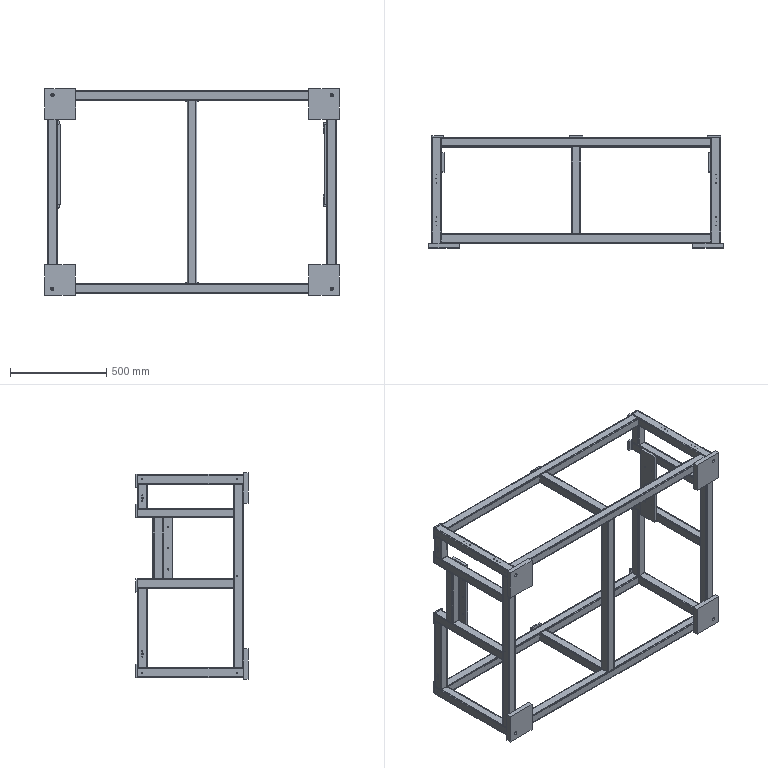Part | NX | features BREP 37 | 37 solids | 722 faces | box 1533 x 583 x 1076 mm | volume 11117929 mm3 | cylinder 395 | plane 327 | commonest cylinder face diameters 10 x103 3.3 x96 5 x92 6.8 x60 14 x36 17.5 x8